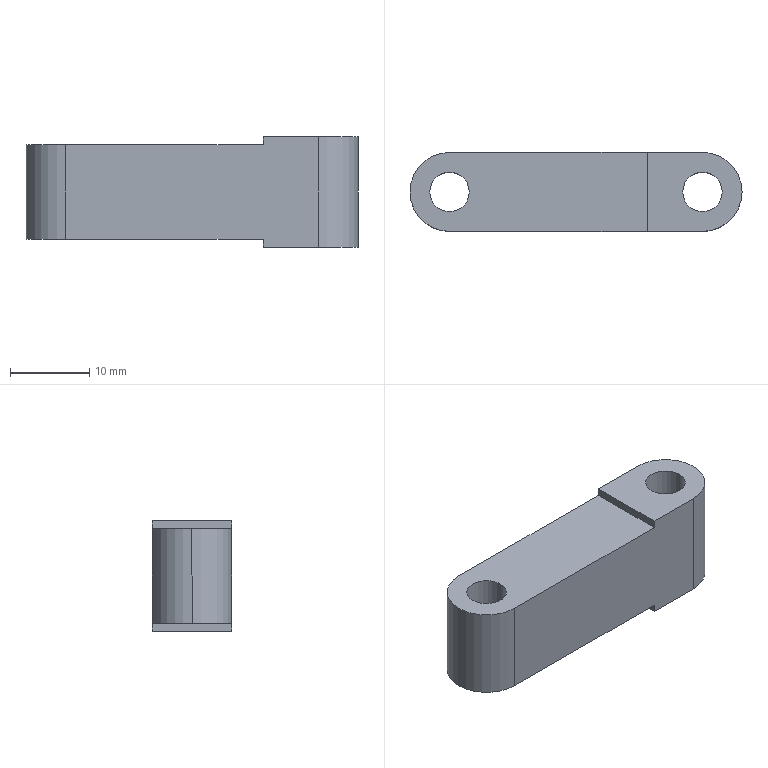Part | STEP file | gripper arm 2_default | 1 solid | 16 faces | box 42 x 10 x 14 mm | volume 4491 mm3 | cylinder 8 | plane 8 | commonest cylinder face diameters 5 x4 10 x4
STEP:
#1=CARTESIAN_POINT('',(0.,0.,0.));
#2=DIRECTION('',(0.,0.,1.));
#3=DIRECTION('',(1.,0.,0.));
#4=AXIS2_PLACEMENT_3D('',#1,#2,#3);
#5=CARTESIAN_POINT('',(18.5,0.,0.));
#6=VERTEX_POINT('',#5);
#7=CARTESIAN_POINT('',(18.5,0.,14.));
#8=VERTEX_POINT('',#7);
#9=CARTESIAN_POINT('',(18.5,0.,0.));
#10=DIRECTION('',(0.,0.,1.));
#11=VECTOR('',#10,1.);
#12=LINE('',#9,#11);
#13=CARTESIAN_POINT('',(16.,0.,0.));
#14=DIRECTION('',(0.,0.,1.));
#15=DIRECTION('',(1.,0.,0.));
#16=AXIS2_PLACEMENT_3D('',#13,#14,#15);
#17=CYLINDRICAL_SURFACE('',#16,2.5);
#18=CARTESIAN_POINT('',(6.283,0.));
#19=DIRECTION('',(0.,1.));
#20=VECTOR('',#19,1.);
#21=LINE('',#18,#20);
#22=(GEOMETRIC_REPRESENTATION_CONTEXT(2)PARAMETRIC_REPRESENTATION_CONTEXT()REPRESENTATION_CONTEXT('',''));
#23=DEFINITIONAL_REPRESENTATION('',(#21),#22);
#24=PCURVE('',#17,#23);
#25=CARTESIAN_POINT('',(16.,0.,0.));
#26=DIRECTION('',(0.,0.,1.));
#27=DIRECTION('',(1.,0.,0.));
#28=AXIS2_PLACEMENT_3D('',#25,#26,#27);
#29=CYLINDRICAL_SURFACE('',#28,2.5);
#30=CARTESIAN_POINT('',(0.,0.));
#31=DIRECTION('',(0.,1.));
#32=VECTOR('',#31,1.);
#33=LINE('',#30,#32);
#34=(GEOMETRIC_REPRESENTATION_CONTEXT(2)PARAMETRIC_REPRESENTATION_CONTEXT()REPRESENTATION_CONTEXT('',''));
#35=DEFINITIONAL_REPRESENTATION('',(#33),#34);
#36=PCURVE('',#29,#35);
#37=SURFACE_CURVE('',#12,(#24,#36),.PCURVE_S1.);
#38=EDGE_CURVE('',#6,#8,#37,.T.);
#39=ORIENTED_EDGE('',*,*,#38,.T.);
#40=CARTESIAN_POINT('',(13.5,0.,14.));
#41=VERTEX_POINT('',#40);
#42=CARTESIAN_POINT('',(16.,0.,14.));
#43=DIRECTION('',(0.,0.,1.));
#44=DIRECTION('',(1.,0.,0.));
#45=AXIS2_PLACEMENT_3D('',#42,#43,#44);
#46=CIRCLE('',#45,2.5);
#47=CARTESIAN_POINT('',(0.,14.));
#48=DIRECTION('',(1.,0.));
#49=VECTOR('',#48,1.);
#50=LINE('',#47,#49);
#51=(GEOMETRIC_REPRESENTATION_CONTEXT(2)PARAMETRIC_REPRESENTATION_CONTEXT()REPRESENTATION_CONTEXT('',''));
#52=DEFINITIONAL_REPRESENTATION('',(#50),#51);
#53=PCURVE('',#17,#52);
#54=CARTESIAN_POINT('',(0.,0.,14.));
#55=DIRECTION('',(0.,0.,1.));
#56=DIRECTION('',(1.,0.,0.));
#57=AXIS2_PLACEMENT_3D('',#54,#55,#56);
#58=PLANE('',#57);
#59=CARTESIAN_POINT('',(16.,0.));
#60=DIRECTION('',(1.,0.));
#61=AXIS2_PLACEMENT_2D('',#59,#60);
#62=CIRCLE('',#61,2.5);
#63=(GEOMETRIC_REPRESENTATION_CONTEXT(2)PARAMETRIC_REPRESENTATION_CONTEXT()REPRESENTATION_CONTEXT('',''));
#64=DEFINITIONAL_REPRESENTATION('',(#62),#63);
#65=PCURVE('',#58,#64);
#66=SURFACE_CURVE('',#46,(#53,#65),.PCURVE_S1.);
#67=EDGE_CURVE('',#41,#8,#66,.T.);
#68=ORIENTED_EDGE('',*,*,#67,.F.);
#69=CARTESIAN_POINT('',(13.5,0.,0.));
#70=VERTEX_POINT('',#69);
#71=CARTESIAN_POINT('',(13.5,0.,0.));
#72=DIRECTION('',(0.,0.,1.));
#73=VECTOR('',#72,1.);
#74=LINE('',#71,#73);
#75=CARTESIAN_POINT('',(3.142,0.));
#76=DIRECTION('',(0.,1.));
#77=VECTOR('',#76,1.);
#78=LINE('',#75,#77);
#79=(GEOMETRIC_REPRESENTATION_CONTEXT(2)PARAMETRIC_REPRESENTATION_CONTEXT()REPRESENTATION_CONTEXT('',''));
#80=DEFINITIONAL_REPRESENTATION('',(#78),#79);
#81=PCURVE('',#17,#80);
#82=CARTESIAN_POINT('',(3.142,0.));
#83=DIRECTION('',(0.,1.));
#84=VECTOR('',#83,1.);
#85=LINE('',#82,#84);
#86=(GEOMETRIC_REPRESENTATION_CONTEXT(2)PARAMETRIC_REPRESENTATION_CONTEXT()REPRESENTATION_CONTEXT('',''));
#87=DEFINITIONAL_REPRESENTATION('',(#85),#86);
#88=PCURVE('',#29,#87);
#89=SURFACE_CURVE('',#74,(#81,#88),.PCURVE_S1.);
#90=EDGE_CURVE('',#70,#41,#89,.T.);
#91=ORIENTED_EDGE('',*,*,#90,.F.);
#92=CARTESIAN_POINT('',(16.,0.,0.));
#93=DIRECTION('',(0.,0.,1.));
#94=DIRECTION('',(1.,0.,0.));
#95=AXIS2_PLACEMENT_3D('',#92,#93,#94);
#96=CIRCLE('',#95,2.5);
#97=CARTESIAN_POINT('',(0.,0.));
#98=DIRECTION('',(1.,0.));
#99=VECTOR('',#98,1.);
#100=LINE('',#97,#99);
#101=(GEOMETRIC_REPRESENTATION_CONTEXT(2)PARAMETRIC_REPRESENTATION_CONTEXT()REPRESENTATION_CONTEXT('',''));
#102=DEFINITIONAL_REPRESENTATION('',(#100),#101);
#103=PCURVE('',#17,#102);
#104=CARTESIAN_POINT('',(0.,0.,0.));
#105=DIRECTION('',(0.,0.,1.));
#106=DIRECTION('',(1.,0.,0.));
#107=AXIS2_PLACEMENT_3D('',#104,#105,#106);
#108=PLANE('',#107);
#109=CARTESIAN_POINT('',(16.,0.));
#110=DIRECTION('',(1.,0.));
#111=AXIS2_PLACEMENT_2D('',#109,#110);
#112=CIRCLE('',#111,2.5);
#113=(GEOMETRIC_REPRESENTATION_CONTEXT(2)PARAMETRIC_REPRESENTATION_CONTEXT()REPRESENTATION_CONTEXT('',''));
#114=DEFINITIONAL_REPRESENTATION('',(#112),#113);
#115=PCURVE('',#108,#114);
#116=SURFACE_CURVE('',#96,(#103,#115),.PCURVE_S1.);
#117=EDGE_CURVE('',#70,#6,#116,.T.);
#118=ORIENTED_EDGE('',*,*,#117,.T.);
#119=EDGE_LOOP('',(#39,#68,#91,#118));
#120=FACE_BOUND('',#119,.F.);
#121=ADVANCED_FACE('',(#120),#17,.F.);
#122=CARTESIAN_POINT('',(-13.5,0.,1.));
#123=VERTEX_POINT('',#122);
#124=CARTESIAN_POINT('',(-13.5,0.,13.));
#125=VERTEX_POINT('',#124);
#126=CARTESIAN_POINT('',(-13.5,0.,0.));
#127=DIRECTION('',(0.,0.,1.));
#128=VECTOR('',#127,1.);
#129=LINE('',#126,#128);
#130=CARTESIAN_POINT('',(-16.,0.,0.));
#131=DIRECTION('',(0.,0.,1.));
#132=DIRECTION('',(1.,0.,0.));
#133=AXIS2_PLACEMENT_3D('',#130,#131,#132);
#134=CYLINDRICAL_SURFACE('',#133,2.5);
#135=CARTESIAN_POINT('',(6.283,0.));
#136=DIRECTION('',(0.,1.));
#137=VECTOR('',#136,1.);
#138=LINE('',#135,#137);
#139=(GEOMETRIC_REPRESENTATION_CONTEXT(2)PARAMETRIC_REPRESENTATION_CONTEXT()REPRESENTATION_CONTEXT('',''));
#140=DEFINITIONAL_REPRESENTATION('',(#138),#139);
#141=PCURVE('',#134,#140);
#142=CARTESIAN_POINT('',(-16.,0.,0.));
#143=DIRECTION('',(0.,0.,1.));
#144=DIRECTION('',(1.,0.,0.));
#145=AXIS2_PLACEMENT_3D('',#142,#143,#144);
#146=CYLINDRICAL_SURFACE('',#145,2.5);
#147=CARTESIAN_POINT('',(0.,0.));
#148=DIRECTION('',(0.,1.));
#149=VECTOR('',#148,1.);
#150=LINE('',#147,#149);
#151=(GEOMETRIC_REPRESENTATION_CONTEXT(2)PARAMETRIC_REPRESENTATION_CONTEXT()REPRESENTATION_CONTEXT('',''));
#152=DEFINITIONAL_REPRESENTATION('',(#150),#151);
#153=PCURVE('',#146,#152);
#154=SURFACE_CURVE('',#129,(#141,#153),.PCURVE_S1.);
#155=EDGE_CURVE('',#123,#125,#154,.T.);
#156=ORIENTED_EDGE('',*,*,#155,.T.);
#157=CARTESIAN_POINT('',(-18.5,0.,13.));
#158=VERTEX_POINT('',#157);
#159=CARTESIAN_POINT('',(-16.,0.,13.));
#160=DIRECTION('',(0.,0.,-1.));
#161=DIRECTION('',(1.,0.,0.));
#162=AXIS2_PLACEMENT_3D('',#159,#160,#161);
#163=CIRCLE('',#162,2.5);
#164=CARTESIAN_POINT('',(6.283,13.));
#165=DIRECTION('',(-1.,0.));
#166=VECTOR('',#165,1.);
#167=LINE('',#164,#166);
#168=(GEOMETRIC_REPRESENTATION_CONTEXT(2)PARAMETRIC_REPRESENTATION_CONTEXT()REPRESENTATION_CONTEXT('',''));
#169=DEFINITIONAL_REPRESENTATION('',(#167),#168);
#170=PCURVE('',#134,#169);
#171=CARTESIAN_POINT('',(0.,0.,13.));
#172=DIRECTION('',(0.,0.,1.));
#173=DIRECTION('',(1.,0.,0.));
#174=AXIS2_PLACEMENT_3D('',#171,#172,#173);
#175=PLANE('',#174);
#176=CARTESIAN_POINT('',(-13.5,0.));
#177=CARTESIAN_POINT('',(-13.5,-4.33));
#178=CARTESIAN_POINT('',(-17.25,-2.165));
#179=CARTESIAN_POINT('',(-21.,0.));
#180=CARTESIAN_POINT('',(-17.25,2.165));
#181=CARTESIAN_POINT('',(-13.5,4.33));
#182=CARTESIAN_POINT('',(-13.5,0.));
#183=(BOUNDED_CURVE()B_SPLINE_CURVE(2,(#176,#177,#178,#179,#180,#181,#182),.UNSPECIFIED.,.T.,.F.)B_SPLINE_CURVE_WITH_KNOTS((1,2,2,2,2,1),(-2.094,0.,2.094,4.189,6.283,8.378),.UNSPECIFIED.)CURVE()GEOMETRIC_REPRESENTATION_ITEM()RATIONAL_B_SPLINE_CURVE((1.,0.5,1.,0.5,1.,0.5,1.))REPRESENTATION_ITEM(''));
#184=(GEOMETRIC_REPRESENTATION_CONTEXT(2)PARAMETRIC_REPRESENTATION_CONTEXT()REPRESENTATION_CONTEXT('',''));
#185=DEFINITIONAL_REPRESENTATION('',(#183),#184);
#186=PCURVE('',#175,#185);
#187=SURFACE_CURVE('',#163,(#170,#186),.PCURVE_S1.);
#188=EDGE_CURVE('',#125,#158,#187,.T.);
#189=ORIENTED_EDGE('',*,*,#188,.T.);
#190=CARTESIAN_POINT('',(-18.5,0.,1.));
#191=VERTEX_POINT('',#190);
#192=CARTESIAN_POINT('',(-18.5,0.,0.));
#193=DIRECTION('',(0.,0.,1.));
#194=VECTOR('',#193,1.);
#195=LINE('',#192,#194);
#196=CARTESIAN_POINT('',(3.142,0.));
#197=DIRECTION('',(0.,1.));
#198=VECTOR('',#197,1.);
#199=LINE('',#196,#198);
#200=(GEOMETRIC_REPRESENTATION_CONTEXT(2)PARAMETRIC_REPRESENTATION_CONTEXT()REPRESENTATION_CONTEXT('',''));
#201=DEFINITIONAL_REPRESENTATION('',(#199),#200);
#202=PCURVE('',#134,#201);
#203=CARTESIAN_POINT('',(3.142,0.));
#204=DIRECTION('',(0.,1.));
#205=VECTOR('',#204,1.);
#206=LINE('',#203,#205);
#207=(GEOMETRIC_REPRESENTATION_CONTEXT(2)PARAMETRIC_REPRESENTATION_CONTEXT()REPRESENTATION_CONTEXT('',''));
#208=DEFINITIONAL_REPRESENTATION('',(#206),#207);
#209=PCURVE('',#146,#208);
#210=SURFACE_CURVE('',#195,(#202,#209),.PCURVE_S1.);
#211=EDGE_CURVE('',#191,#158,#210,.T.);
#212=ORIENTED_EDGE('',*,*,#211,.F.);
#213=CARTESIAN_POINT('',(-16.,0.,1.));
#214=DIRECTION('',(0.,0.,1.));
#215=DIRECTION('',(-1.,0.,0.));
#216=AXIS2_PLACEMENT_3D('',#213,#214,#215);
#217=CIRCLE('',#216,2.5);
#218=CARTESIAN_POINT('',(3.142,1.));
#219=DIRECTION('',(1.,0.));
#220=VECTOR('',#219,1.);
#221=LINE('',#218,#220);
#222=(GEOMETRIC_REPRESENTATION_CONTEXT(2)PARAMETRIC_REPRESENTATION_CONTEXT()REPRESENTATION_CONTEXT('',''));
#223=DEFINITIONAL_REPRESENTATION('',(#221),#222);
#224=PCURVE('',#134,#223);
#225=CARTESIAN_POINT('',(0.,0.,1.));
#226=DIRECTION('',(0.,0.,-1.));
#227=DIRECTION('',(-1.,0.,0.));
#228=AXIS2_PLACEMENT_3D('',#225,#226,#227);
#229=PLANE('',#228);
#230=CARTESIAN_POINT('',(18.5,0.));
#231=CARTESIAN_POINT('',(18.5,-4.33));
#232=CARTESIAN_POINT('',(14.75,-2.165));
#233=CARTESIAN_POINT('',(11.,0.));
#234=CARTESIAN_POINT('',(14.75,2.165));
#235=CARTESIAN_POINT('',(18.5,4.33));
#236=CARTESIAN_POINT('',(18.5,0.));
#237=(BOUNDED_CURVE()B_SPLINE_CURVE(2,(#230,#231,#232,#233,#234,#235,#236),.UNSPECIFIED.,.T.,.F.)B_SPLINE_CURVE_WITH_KNOTS((1,2,2,2,2,1),(-2.094,0.,2.094,4.189,6.283,8.378),.UNSPECIFIED.)CURVE()GEOMETRIC_REPRESENTATION_ITEM()RATIONAL_B_SPLINE_CURVE((1.,0.5,1.,0.5,1.,0.5,1.))REPRESENTATION_ITEM(''));
#238=(GEOMETRIC_REPRESENTATION_CONTEXT(2)PARAMETRIC_REPRESENTATION_CONTEXT()REPRESENTATION_CONTEXT('',''));
#239=DEFINITIONAL_REPRESENTATION('',(#237),#238);
#240=PCURVE('',#229,#239);
#241=SURFACE_CURVE('',#217,(#224,#240),.PCURVE_S1.);
#242=EDGE_CURVE('',#191,#123,#241,.T.);
#243=ORIENTED_EDGE('',*,*,#242,.T.);
#244=EDGE_LOOP('',(#156,#189,#212,#243));
#245=FACE_BOUND('',#244,.F.);
#246=ADVANCED_FACE('',(#245),#134,.F.);
#247=CARTESIAN_POINT('',(-16.,0.,13.));
#248=DIRECTION('',(0.,0.,-1.));
#249=DIRECTION('',(1.,0.,0.));
#250=AXIS2_PLACEMENT_3D('',#247,#248,#249);
#251=CIRCLE('',#250,2.5);
#252=CARTESIAN_POINT('',(6.283,13.));
#253=DIRECTION('',(-1.,0.));
#254=VECTOR('',#253,1.);
#255=LINE('',#252,#254);
#256=(GEOMETRIC_REPRESENTATION_CONTEXT(2)PARAMETRIC_REPRESENTATION_CONTEXT()REPRESENTATION_CONTEXT('',''));
#257=DEFINITIONAL_REPRESENTATION('',(#255),#256);
#258=PCURVE('',#146,#257);
#259=CARTESIAN_POINT('',(-13.5,0.));
#260=CARTESIAN_POINT('',(-13.5,-4.33));
#261=CARTESIAN_POINT('',(-17.25,-2.165));
#262=CARTESIAN_POINT('',(-21.,0.));
#263=CARTESIAN_POINT('',(-17.25,2.165));
#264=CARTESIAN_POINT('',(-13.5,4.33));
#265=CARTESIAN_POINT('',(-13.5,0.));
#266=(BOUNDED_CURVE()B_SPLINE_CURVE(2,(#259,#260,#261,#262,#263,#264,#265),.UNSPECIFIED.,.T.,.F.)B_SPLINE_CURVE_WITH_KNOTS((1,2,2,2,2,1),(-2.094,0.,2.094,4.189,6.283,8.378),.UNSPECIFIED.)CURVE()GEOMETRIC_REPRESENTATION_ITEM()RATIONAL_B_SPLINE_CURVE((1.,0.5,1.,0.5,1.,0.5,1.))REPRESENTATION_ITEM(''));
#267=(GEOMETRIC_REPRESENTATION_CONTEXT(2)PARAMETRIC_REPRESENTATION_CONTEXT()REPRESENTATION_CONTEXT('',''));
#268=DEFINITIONAL_REPRESENTATION('',(#266),#267);
#269=PCURVE('',#175,#268);
#270=SURFACE_CURVE('',#251,(#258,#269),.PCURVE_S1.);
#271=EDGE_CURVE('',#158,#125,#270,.T.);
#272=ORIENTED_EDGE('',*,*,#271,.T.);
#273=ORIENTED_EDGE('',*,*,#155,.F.);
#274=CARTESIAN_POINT('',(-16.,0.,1.));
#275=DIRECTION('',(0.,0.,1.));
#276=DIRECTION('',(-1.,0.,0.));
#277=AXIS2_PLACEMENT_3D('',#274,#275,#276);
#278=CIRCLE('',#277,2.5);
#279=CARTESIAN_POINT('',(-3.142,1.));
#280=DIRECTION('',(1.,0.));
#281=VECTOR('',#280,1.);
#282=LINE('',#279,#281);
#283=(GEOMETRIC_REPRESENTATION_CONTEXT(2)PARAMETRIC_REPRESENTATION_CONTEXT()REPRESENTATION_CONTEXT('',''));
#284=DEFINITIONAL_REPRESENTATION('',(#282),#283);
#285=PCURVE('',#146,#284);
#286=CARTESIAN_POINT('',(18.5,0.));
#287=CARTESIAN_POINT('',(18.5,-4.33));
#288=CARTESIAN_POINT('',(14.75,-2.165));
#289=CARTESIAN_POINT('',(11.,0.));
#290=CARTESIAN_POINT('',(14.75,2.165));
#291=CARTESIAN_POINT('',(18.5,4.33));
#292=CARTESIAN_POINT('',(18.5,0.));
#293=(BOUNDED_CURVE()B_SPLINE_CURVE(2,(#286,#287,#288,#289,#290,#291,#292),.UNSPECIFIED.,.T.,.F.)B_SPLINE_CURVE_WITH_KNOTS((1,2,2,2,2,1),(-2.094,0.,2.094,4.189,6.283,8.378),.UNSPECIFIED.)CURVE()GEOMETRIC_REPRESENTATION_ITEM()RATIONAL_B_SPLINE_CURVE((1.,0.5,1.,0.5,1.,0.5,1.))REPRESENTATION_ITEM(''));
#294=(GEOMETRIC_REPRESENTATION_CONTEXT(2)PARAMETRIC_REPRESENTATION_CONTEXT()REPRESENTATION_CONTEXT('',''));
#295=DEFINITIONAL_REPRESENTATION('',(#293),#294);
#296=PCURVE('',#229,#295);
#297=SURFACE_CURVE('',#278,(#285,#296),.PCURVE_S1.);
#298=EDGE_CURVE('',#123,#191,#297,.T.);
#299=ORIENTED_EDGE('',*,*,#298,.T.);
#300=ORIENTED_EDGE('',*,*,#211,.T.);
#301=EDGE_LOOP('',(#272,#273,#299,#300));
#302=FACE_BOUND('',#301,.F.);
#303=ADVANCED_FACE('',(#302),#146,.F.);
#304=CARTESIAN_POINT('',(-16.,5.,1.));
#305=VERTEX_POINT('',#304);
#306=CARTESIAN_POINT('',(-16.,5.,13.));
#307=VERTEX_POINT('',#306);
#308=CARTESIAN_POINT('',(-16.,5.,14.));
#309=DIRECTION('',(0.,0.,1.));
#310=VECTOR('',#309,1.);
#311=LINE('',#308,#310);
#312=CARTESIAN_POINT('',(-16.,0.,14.));
#313=DIRECTION('',(0.,0.,-1.));
#314=DIRECTION('',(-1.,0.,0.));
#315=AXIS2_PLACEMENT_3D('',#312,#313,#314);
#316=CYLINDRICAL_SURFACE('',#315,5.);
#317=CARTESIAN_POINT('',(1.571,0.));
#318=DIRECTION('',(0.,-1.));
#319=VECTOR('',#318,1.);
#320=LINE('',#317,#319);
#321=(GEOMETRIC_REPRESENTATION_CONTEXT(2)PARAMETRIC_REPRESENTATION_CONTEXT()REPRESENTATION_CONTEXT('',''));
#322=DEFINITIONAL_REPRESENTATION('',(#320),#321);
#323=PCURVE('',#316,#322);
#324=CARTESIAN_POINT('',(-21.,5.,14.));
#325=DIRECTION('',(0.,-1.,0.));
#326=DIRECTION('',(0.,0.,-1.));
#327=AXIS2_PLACEMENT_3D('',#324,#325,#326);
#328=PLANE('',#327);
#329=CARTESIAN_POINT('',(0.,5.));
#330=DIRECTION('',(-1.,0.));
#331=VECTOR('',#330,1.);
#332=LINE('',#329,#331);
#333=(GEOMETRIC_REPRESENTATION_CONTEXT(2)PARAMETRIC_REPRESENTATION_CONTEXT()REPRESENTATION_CONTEXT('',''));
#334=DEFINITIONAL_REPRESENTATION('',(#332),#333);
#335=PCURVE('',#328,#334);
#336=SURFACE_CURVE('',#311,(#323,#335),.PCURVE_S1.);
#337=EDGE_CURVE('',#305,#307,#336,.T.);
#338=ORIENTED_EDGE('',*,*,#337,.F.);
#339=CARTESIAN_POINT('',(-21.,0.,1.));
#340=VERTEX_POINT('',#339);
#341=CARTESIAN_POINT('',(-16.,0.,1.));
#342=DIRECTION('',(0.,0.,1.));
#343=DIRECTION('',(-1.,0.,0.));
#344=AXIS2_PLACEMENT_3D('',#341,#342,#343);
#345=CIRCLE('',#344,5.);
#346=CARTESIAN_POINT('',(6.283,13.));
#347=DIRECTION('',(-1.,0.));
#348=VECTOR('',#347,1.);
#349=LINE('',#346,#348);
#350=(GEOMETRIC_REPRESENTATION_CONTEXT(2)PARAMETRIC_REPRESENTATION_CONTEXT()REPRESENTATION_CONTEXT('',''));
#351=DEFINITIONAL_REPRESENTATION('',(#349),#350);
#352=PCURVE('',#316,#351);
#353=CARTESIAN_POINT('',(21.,0.));
#354=CARTESIAN_POINT('',(21.,-8.66));
#355=CARTESIAN_POINT('',(13.5,-4.33));
#356=CARTESIAN_POINT('',(6.,0.));
#357=CARTESIAN_POINT('',(13.5,4.33));
#358=CARTESIAN_POINT('',(21.,8.66));
#359=CARTESIAN_POINT('',(21.,0.));
#360=(BOUNDED_CURVE()B_SPLINE_CURVE(2,(#353,#354,#355,#356,#357,#358,#359),.UNSPECIFIED.,.T.,.F.)B_SPLINE_CURVE_WITH_KNOTS((1,2,2,2,2,1),(-2.094,0.,2.094,4.189,6.283,8.378),.UNSPECIFIED.)CURVE()GEOMETRIC_REPRESENTATION_ITEM()RATIONAL_B_SPLINE_CURVE((1.,0.5,1.,0.5,1.,0.5,1.))REPRESENTATION_ITEM(''));
#361=(GEOMETRIC_REPRESENTATION_CONTEXT(2)PARAMETRIC_REPRESENTATION_CONTEXT()REPRESENTATION_CONTEXT('',''));
#362=DEFINITIONAL_REPRESENTATION('',(#360),#361);
#363=PCURVE('',#229,#362);
#364=SURFACE_CURVE('',#345,(#352,#363),.PCURVE_S1.);
#365=EDGE_CURVE('',#305,#340,#364,.T.);
#366=ORIENTED_EDGE('',*,*,#365,.T.);
#367=CARTESIAN_POINT('',(-21.,0.,13.));
#368=VERTEX_POINT('',#367);
#369=CARTESIAN_POINT('',(-21.,0.,14.));
#370=DIRECTION('',(0.,0.,-1.));
#371=VECTOR('',#370,1.);
#372=LINE('',#369,#371);
#373=CARTESIAN_POINT('',(0.,0.));
#374=DIRECTION('',(0.,1.));
#375=VECTOR('',#374,1.);
#376=LINE('',#373,#375);
#377=(GEOMETRIC_REPRESENTATION_CONTEXT(2)PARAMETRIC_REPRESENTATION_CONTEXT()REPRESENTATION_CONTEXT('',''));
#378=DEFINITIONAL_REPRESENTATION('',(#376),#377);
#379=PCURVE('',#316,#378);
#380=CARTESIAN_POINT('',(-16.,0.,14.));
#381=DIRECTION('',(0.,0.,-1.));
#382=DIRECTION('',(-1.,0.,0.));
#383=AXIS2_PLACEMENT_3D('',#380,#381,#382);
#384=CYLINDRICAL_SURFACE('',#383,5.);
#385=CARTESIAN_POINT('',(6.283,0.));
#386=DIRECTION('',(0.,1.));
#387=VECTOR('',#386,1.);
#388=LINE('',#385,#387);
#389=(GEOMETRIC_REPRESENTATION_CONTEXT(2)PARAMETRIC_REPRESENTATION_CONTEXT()REPRESENTATION_CONTEXT('',''));
#390=DEFINITIONAL_REPRESENTATION('',(#388),#389);
#391=PCURVE('',#384,#390);
#392=SURFACE_CURVE('',#372,(#379,#391),.PCURVE_S1.);
#393=EDGE_CURVE('',#368,#340,#392,.T.);
#394=ORIENTED_EDGE('',*,*,#393,.F.);
#395=CARTESIAN_POINT('',(-16.,0.,13.));
#396=DIRECTION('',(0.,0.,-1.));
#397=DIRECTION('',(1.,0.,0.));
#398=AXIS2_PLACEMENT_3D('',#395,#396,#397);
#399=CIRCLE('',#398,5.);
#400=CARTESIAN_POINT('',(-3.142,1.));
#401=DIRECTION('',(1.,0.));
#402=VECTOR('',#401,1.);
#403=LINE('',#400,#402);
#404=(GEOMETRIC_REPRESENTATION_CONTEXT(2)PARAMETRIC_REPRESENTATION_CONTEXT()REPRESENTATION_CONTEXT('',''));
#405=DEFINITIONAL_REPRESENTATION('',(#403),#404);
#406=PCURVE('',#316,#405);
#407=CARTESIAN_POINT('',(-11.,0.));
#408=CARTESIAN_POINT('',(-11.,-8.66));
#409=CARTESIAN_POINT('',(-18.5,-4.33));
#410=CARTESIAN_POINT('',(-26.,0.));
#411=CARTESIAN_POINT('',(-18.5,4.33));
#412=CARTESIAN_POINT('',(-11.,8.66));
#413=CARTESIAN_POINT('',(-11.,0.));
#414=(BOUNDED_CURVE()B_SPLINE_CURVE(2,(#407,#408,#409,#410,#411,#412,#413),.UNSPECIFIED.,.T.,.F.)B_SPLINE_CURVE_WITH_KNOTS((1,2,2,2,2,1),(-2.094,0.,2.094,4.189,6.283,8.378),.UNSPECIFIED.)CURVE()GEOMETRIC_REPRESENTATION_ITEM()RATIONAL_B_SPLINE_CURVE((1.,0.5,1.,0.5,1.,0.5,1.))REPRESENTATION_ITEM(''));
#415=(GEOMETRIC_REPRESENTATION_CONTEXT(2)PARAMETRIC_REPRESENTATION_CONTEXT()REPRESENTATION_CONTEXT('',''));
#416=DEFINITIONAL_REPRESENTATION('',(#414),#415);
#417=PCURVE('',#175,#416);
#418=SURFACE_CURVE('',#399,(#406,#417),.PCURVE_S1.);
#419=EDGE_CURVE('',#368,#307,#418,.T.);
#420=ORIENTED_EDGE('',*,*,#419,.T.);
#421=EDGE_LOOP('',(#338,#366,#394,#420));
#422=FACE_BOUND('',#421,.T.);
#423=ADVANCED_FACE('',(#422),#316,.T.);
#424=ORIENTED_EDGE('',*,*,#393,.T.);
#425=CARTESIAN_POINT('',(-16.,-5.,1.));
#426=VERTEX_POINT('',#425);
#427=CARTESIAN_POINT('',(-16.,0.,1.));
#428=DIRECTION('',(0.,0.,1.));
#429=DIRECTION('',(-1.,0.,0.));
#430=AXIS2_PLACEMENT_3D('',#427,#428,#429);
#431=CIRCLE('',#430,5.);
#432=CARTESIAN_POINT('',(6.283,13.));
#433=DIRECTION('',(-1.,0.));
#434=VECTOR('',#433,1.);
#435=LINE('',#432,#434);
#436=(GEOMETRIC_REPRESENTATION_CONTEXT(2)PARAMETRIC_REPRESENTATION_CONTEXT()REPRESENTATION_CONTEXT('',''));
#437=DEFINITIONAL_REPRESENTATION('',(#435),#436);
#438=PCURVE('',#384,#437);
#439=CARTESIAN_POINT('',(21.,0.));
#440=CARTESIAN_POINT('',(21.,-8.66));
#441=CARTESIAN_POINT('',(13.5,-4.33));
#442=CARTESIAN_POINT('',(6.,0.));
#443=CARTESIAN_POINT('',(13.5,4.33));
#444=CARTESIAN_POINT('',(21.,8.66));
#445=CARTESIAN_POINT('',(21.,0.));
#446=(BOUNDED_CURVE()B_SPLINE_CURVE(2,(#439,#440,#441,#442,#443,#444,#445),.UNSPECIFIED.,.T.,.F.)B_SPLINE_CURVE_WITH_KNOTS((1,2,2,2,2,1),(-2.094,0.,2.094,4.189,6.283,8.378),.UNSPECIFIED.)CURVE()GEOMETRIC_REPRESENTATION_ITEM()RATIONAL_B_SPLINE_CURVE((1.,0.5,1.,0.5,1.,0.5,1.))REPRESENTATION_ITEM(''));
#447=(GEOMETRIC_REPRESENTATION_CONTEXT(2)PARAMETRIC_REPRESENTATION_CONTEXT()REPRESENTATION_CONTEXT('',''));
#448=DEFINITIONAL_REPRESENTATION('',(#446),#447);
#449=PCURVE('',#229,#448);
#450=SURFACE_CURVE('',#431,(#438,#449),.PCURVE_S1.);
#451=EDGE_CURVE('',#340,#426,#450,.T.);
#452=ORIENTED_EDGE('',*,*,#451,.T.);
#453=CARTESIAN_POINT('',(-16.,-5.,13.));
#454=VERTEX_POINT('',#453);
#455=CARTESIAN_POINT('',(-16.,-5.,14.));
#456=DIRECTION('',(0.,0.,-1.));
#457=VECTOR('',#456,1.);
#458=LINE('',#455,#457);
#459=CARTESIAN_POINT('',(4.712,0.));
#460=DIRECTION('',(0.,1.));
#461=VECTOR('',#460,1.);
#462=LINE('',#459,#461);
#463=(GEOMETRIC_REPRESENTATION_CONTEXT(2)PARAMETRIC_REPRESENTATION_CONTEXT()REPRESENTATION_CONTEXT('',''));
#464=DEFINITIONAL_REPRESENTATION('',(#462),#463);
#465=PCURVE('',#384,#464);
#466=CARTESIAN_POINT('',(-21.,-5.,14.));
#467=DIRECTION('',(0.,1.,0.));
#468=DIRECTION('',(0.,0.,1.));
#469=AXIS2_PLACEMENT_3D('',#466,#467,#468);
#470=PLANE('',#469);
#471=CARTESIAN_POINT('',(0.,5.));
#472=DIRECTION('',(-1.,0.));
#473=VECTOR('',#472,1.);
#474=LINE('',#471,#473);
#475=(GEOMETRIC_REPRESENTATION_CONTEXT(2)PARAMETRIC_REPRESENTATION_CONTEXT()REPRESENTATION_CONTEXT('',''));
#476=DEFINITIONAL_REPRESENTATION('',(#474),#475);
#477=PCURVE('',#470,#476);
#478=SURFACE_CURVE('',#458,(#465,#477),.PCURVE_S1.);
#479=EDGE_CURVE('',#454,#426,#478,.T.);
#480=ORIENTED_EDGE('',*,*,#479,.F.);
#481=CARTESIAN_POINT('',(-16.,0.,13.));
#482=DIRECTION('',(0.,0.,-1.));
#483=DIRECTION('',(1.,0.,0.));
#484=AXIS2_PLACEMENT_3D('',#481,#482,#483);
#485=CIRCLE('',#484,5.);
#486=CARTESIAN_POINT('',(3.142,1.));
#487=DIRECTION('',(1.,0.));
#488=VECTOR('',#487,1.);
#489=LINE('',#486,#488);
#490=(GEOMETRIC_REPRESENTATION_CONTEXT(2)PARAMETRIC_REPRESENTATION_CONTEXT()REPRESENTATION_CONTEXT('',''));
#491=DEFINITIONAL_REPRESENTATION('',(#489),#490);
#492=PCURVE('',#384,#491);
#493=CARTESIAN_POINT('',(-11.,0.));
#494=CARTESIAN_POINT('',(-11.,-8.66));
#495=CARTESIAN_POINT('',(-18.5,-4.33));
#496=CARTESIAN_POINT('',(-26.,0.));
#497=CARTESIAN_POINT('',(-18.5,4.33));
#498=CARTESIAN_POINT('',(-11.,8.66));
#499=CARTESIAN_POINT('',(-11.,0.));
#500=(BOUNDED_CURVE()B_SPLINE_CURVE(2,(#493,#494,#495,#496,#497,#498,#499),.UNSPECIFIED.,.T.,.F.)B_SPLINE_CURVE_WITH_KNOTS((1,2,2,2,2,1),(-2.094,0.,2.094,4.189,6.283,8.378),.UNSPECIFIED.)CURVE()GEOMETRIC_REPRESENTATION_ITEM()RATIONAL_B_SPLINE_CURVE((1.,0.5,1.,0.5,1.,0.5,1.))REPRESENTATION_ITEM(''));
#501=(GEOMETRIC_REPRESENTATION_CONTEXT(2)PARAMETRIC_REPRESENTATION_CONTEXT()REPRESENTATION_CONTEXT('',''));
#502=DEFINITIONAL_REPRESENTATION('',(#500),#501);
#503=PCURVE('',#175,#502);
#504=SURFACE_CURVE('',#485,(#492,#503),.PCURVE_S1.);
#505=EDGE_CURVE('',#454,#368,#504,.T.);
#506=ORIENTED_EDGE('',*,*,#505,.T.);
#507=EDGE_LOOP('',(#424,#452,#480,#506));
#508=FACE_BOUND('',#507,.T.);
#509=ADVANCED_FACE('',(#508),#384,.T.);
#510=CARTESIAN_POINT('',(16.,5.,0.));
#511=VERTEX_POINT('',#510);
#512=CARTESIAN_POINT('',(9.,5.,0.));
#513=VERTEX_POINT('',#512);
#514=CARTESIAN_POINT('',(-21.,5.,0.));
#515=DIRECTION('',(-1.,0.,0.));
#516=VECTOR('',#515,1.);
#517=LINE('',#514,#516);
#518=CARTESIAN_POINT('',(14.,0.));
#519=DIRECTION('',(0.,-1.));
#520=VECTOR('',#519,1.);
#521=LINE('',#518,#520);
#522=(GEOMETRIC_REPRESENTATION_CONTEXT(2)PARAMETRIC_REPRESENTATION_CONTEXT()REPRESENTATION_CONTEXT('',''));
#523=DEFINITIONAL_REPRESENTATION('',(#521),#522);
#524=PCURVE('',#328,#523);
#525=CARTESIAN_POINT('',(-21.,5.));
#526=DIRECTION('',(-1.,0.));
#527=VECTOR('',#526,1.);
#528=LINE('',#525,#527);
#529=(GEOMETRIC_REPRESENTATION_CONTEXT(2)PARAMETRIC_REPRESENTATION_CONTEXT()REPRESENTATION_CONTEXT('',''));
#530=DEFINITIONAL_REPRESENTATION('',(#528),#529);
#531=PCURVE('',#108,#530);
#532=SURFACE_CURVE('',#517,(#524,#531),.PCURVE_S1.);
#533=EDGE_CURVE('',#511,#513,#532,.T.);
#534=ORIENTED_EDGE('',*,*,#533,.T.);
#535=CARTESIAN_POINT('',(9.,5.,1.));
#536=VERTEX_POINT('',#535);
#537=CARTESIAN_POINT('',(9.,5.,14.));
#538=DIRECTION('',(0.,0.,1.));
#539=VECTOR('',#538,1.);
#540=LINE('',#537,#539);
#541=CARTESIAN_POINT('',(0.,30.));
#542=DIRECTION('',(-1.,0.));
#543=VECTOR('',#542,1.);
#544=LINE('',#541,#543);
#545=(GEOMETRIC_REPRESENTATION_CONTEXT(2)PARAMETRIC_REPRESENTATION_CONTEXT()REPRESENTATION_CONTEXT('',''));
#546=DEFINITIONAL_REPRESENTATION('',(#544),#545);
#547=PCURVE('',#328,#546);
#548=CARTESIAN_POINT('',(9.,6.326,1.));
#549=DIRECTION('',(1.,0.,0.));
#550=DIRECTION('',(0.,1.,0.));
#551=AXIS2_PLACEMENT_3D('',#548,#549,#550);
#552=PLANE('',#551);
#553=CARTESIAN_POINT('',(-1.326,13.));
#554=DIRECTION('',(0.,1.));
#555=VECTOR('',#554,1.);
#556=LINE('',#553,#555);
#557=(GEOMETRIC_REPRESENTATION_CONTEXT(2)PARAMETRIC_REPRESENTATION_CONTEXT()REPRESENTATION_CONTEXT('',''));
#558=DEFINITIONAL_REPRESENTATION('',(#556),#557);
#559=PCURVE('',#552,#558);
#560=SURFACE_CURVE('',#540,(#547,#559),.PCURVE_S1.);
#561=EDGE_CURVE('',#513,#536,#560,.T.);
#562=ORIENTED_EDGE('',*,*,#561,.T.);
#563=CARTESIAN_POINT('',(-21.,5.,1.));
#564=DIRECTION('',(1.,0.,0.));
#565=VECTOR('',#564,1.);
#566=LINE('',#563,#565);
#567=CARTESIAN_POINT('',(13.,0.));
#568=DIRECTION('',(0.,1.));
#569=VECTOR('',#568,1.);
#570=LINE('',#567,#569);
#571=(GEOMETRIC_REPRESENTATION_CONTEXT(2)PARAMETRIC_REPRESENTATION_CONTEXT()REPRESENTATION_CONTEXT('',''));
#572=DEFINITIONAL_REPRESENTATION('',(#570),#571);
#573=PCURVE('',#328,#572);
#574=CARTESIAN_POINT('',(21.,5.));
#575=DIRECTION('',(-1.,0.));
#576=VECTOR('',#575,1.);
#577=LINE('',#574,#576);
#578=(GEOMETRIC_REPRESENTATION_CONTEXT(2)PARAMETRIC_REPRESENTATION_CONTEXT()REPRESENTATION_CONTEXT('',''));
#579=DEFINITIONAL_REPRESENTATION('',(#577),#578);
#580=PCURVE('',#229,#579);
#581=SURFACE_CURVE('',#566,(#573,#580),.PCURVE_S1.);
#582=EDGE_CURVE('',#305,#536,#581,.T.);
#583=ORIENTED_EDGE('',*,*,#582,.F.);
#584=ORIENTED_EDGE('',*,*,#337,.T.);
#585=CARTESIAN_POINT('',(9.,5.,13.));
#586=VERTEX_POINT('',#585);
#587=CARTESIAN_POINT('',(-21.,5.,13.));
#588=DIRECTION('',(-1.,0.,0.));
#589=VECTOR('',#588,1.);
#590=LINE('',#587,#589);
#591=CARTESIAN_POINT('',(1.,0.));
#592=DIRECTION('',(0.,-1.));
#593=VECTOR('',#592,1.);
#594=LINE('',#591,#593);
#595=(GEOMETRIC_REPRESENTATION_CONTEXT(2)PARAMETRIC_REPRESENTATION_CONTEXT()REPRESENTATION_CONTEXT('',''));
#596=DEFINITIONAL_REPRESENTATION('',(#594),#595);
#597=PCURVE('',#328,#596);
#598=CARTESIAN_POINT('',(-21.,5.));
#599=DIRECTION('',(-1.,0.));
#600=VECTOR('',#599,1.);
#601=LINE('',#598,#600);
#602=(GEOMETRIC_REPRESENTATION_CONTEXT(2)PARAMETRIC_REPRESENTATION_CONTEXT()REPRESENTATION_CONTEXT('',''));
#603=DEFINITIONAL_REPRESENTATION('',(#601),#602);
#604=PCURVE('',#175,#603);
#605=SURFACE_CURVE('',#590,(#597,#604),.PCURVE_S1.);
#606=EDGE_CURVE('',#586,#307,#605,.T.);
#607=ORIENTED_EDGE('',*,*,#606,.F.);
#608=CARTESIAN_POINT('',(9.,5.,14.));
#609=VERTEX_POINT('',#608);
#610=CARTESIAN_POINT('',(9.,5.,14.));
#611=DIRECTION('',(0.,0.,1.));
#612=VECTOR('',#611,1.);
#613=LINE('',#610,#612);
#614=CARTESIAN_POINT('',(0.,30.));
#615=DIRECTION('',(-1.,0.));
#616=VECTOR('',#615,1.);
#617=LINE('',#614,#616);
#618=(GEOMETRIC_REPRESENTATION_CONTEXT(2)PARAMETRIC_REPRESENTATION_CONTEXT()REPRESENTATION_CONTEXT('',''));
#619=DEFINITIONAL_REPRESENTATION('',(#617),#618);
#620=PCURVE('',#328,#619);
#621=CARTESIAN_POINT('',(9.,7.188,13.));
#622=DIRECTION('',(1.,0.,0.));
#623=DIRECTION('',(0.,0.,-1.));
#624=AXIS2_PLACEMENT_3D('',#621,#622,#623);
#625=PLANE('',#624);
#626=CARTESIAN_POINT('',(-1.,-2.188));
#627=DIRECTION('',(-1.,0.));
#628=VECTOR('',#627,1.);
#629=LINE('',#626,#628);
#630=(GEOMETRIC_REPRESENTATION_CONTEXT(2)PARAMETRIC_REPRESENTATION_CONTEXT()REPRESENTATION_CONTEXT('',''));
#631=DEFINITIONAL_REPRESENTATION('',(#629),#630);
#632=PCURVE('',#625,#631);
#633=SURFACE_CURVE('',#613,(#620,#632),.PCURVE_S1.);
#634=EDGE_CURVE('',#586,#609,#633,.T.);
#635=ORIENTED_EDGE('',*,*,#634,.T.);
#636=CARTESIAN_POINT('',(16.,5.,14.));
#637=VERTEX_POINT('',#636);
#638=CARTESIAN_POINT('',(-21.,5.,14.));
#639=DIRECTION('',(-1.,0.,0.));
#640=VECTOR('',#639,1.);
#641=LINE('',#638,#640);
#642=CARTESIAN_POINT('',(0.,0.));
#643=DIRECTION('',(0.,-1.));
#644=VECTOR('',#643,1.);
#645=LINE('',#642,#644);
#646=(GEOMETRIC_REPRESENTATION_CONTEXT(2)PARAMETRIC_REPRESENTATION_CONTEXT()REPRESENTATION_CONTEXT('',''));
#647=DEFINITIONAL_REPRESENTATION('',(#645),#646);
#648=PCURVE('',#328,#647);
#649=CARTESIAN_POINT('',(-21.,5.));
#650=DIRECTION('',(-1.,0.));
#651=VECTOR('',#650,1.);
#652=LINE('',#649,#651);
#653=(GEOMETRIC_REPRESENTATION_CONTEXT(2)PARAMETRIC_REPRESENTATION_CONTEXT()REPRESENTATION_CONTEXT('',''));
#654=DEFINITIONAL_REPRESENTATION('',(#652),#653);
#655=PCURVE('',#58,#654);
#656=SURFACE_CURVE('',#641,(#648,#655),.PCURVE_S1.);
#657=EDGE_CURVE('',#637,#609,#656,.T.);
#658=ORIENTED_EDGE('',*,*,#657,.F.);
#659=CARTESIAN_POINT('',(16.,5.,14.));
#660=DIRECTION('',(0.,0.,-1.));
#661=VECTOR('',#660,1.);
#662=LINE('',#659,#661);
#663=CARTESIAN_POINT('',(0.,37.));
#664=DIRECTION('',(1.,0.));
#665=VECTOR('',#664,1.);
#666=LINE('',#663,#665);
#667=(GEOMETRIC_REPRESENTATION_CONTEXT(2)PARAMETRIC_REPRESENTATION_CONTEXT()REPRESENTATION_CONTEXT('',''));
#668=DEFINITIONAL_REPRESENTATION('',(#666),#667);
#669=PCURVE('',#328,#668);
#670=CARTESIAN_POINT('',(16.,0.,14.));
#671=DIRECTION('',(0.,0.,-1.));
#672=DIRECTION('',(-1.,0.,0.));
#673=AXIS2_PLACEMENT_3D('',#670,#671,#672);
#674=CYLINDRICAL_SURFACE('',#673,5.);
#675=CARTESIAN_POINT('',(1.571,0.));
#676=DIRECTION('',(0.,1.));
#677=VECTOR('',#676,1.);
#678=LINE('',#675,#677);
#679=(GEOMETRIC_REPRESENTATION_CONTEXT(2)PARAMETRIC_REPRESENTATION_CONTEXT()REPRESENTATION_CONTEXT('',''));
#680=DEFINITIONAL_REPRESENTATION('',(#678),#679);
#681=PCURVE('',#674,#680);
#682=SURFACE_CURVE('',#662,(#669,#681),.PCURVE_S1.);
#683=EDGE_CURVE('',#637,#511,#682,.T.);
#684=ORIENTED_EDGE('',*,*,#683,.T.);
#685=EDGE_LOOP('',(#534,#562,#583,#584,#607,#635,#658,#684));
#686=FACE_BOUND('',#685,.T.);
#687=ADVANCED_FACE('',(#686),#328,.F.);
#688=CARTESIAN_POINT('',(9.,-5.,1.));
#689=VERTEX_POINT('',#688);
#690=CARTESIAN_POINT('',(-21.,-5.,1.));
#691=DIRECTION('',(-1.,0.,0.));
#692=VECTOR('',#691,1.);
#693=LINE('',#690,#692);
#694=CARTESIAN_POINT('',(-13.,0.));
#695=DIRECTION('',(0.,-1.));
#696=VECTOR('',#695,1.);
#697=LINE('',#694,#696);
#698=(GEOMETRIC_REPRESENTATION_CONTEXT(2)PARAMETRIC_REPRESENTATION_CONTEXT()REPRESENTATION_CONTEXT('',''));
#699=DEFINITIONAL_REPRESENTATION('',(#697),#698);
#700=PCURVE('',#470,#699);
#701=CARTESIAN_POINT('',(21.,-5.));
#702=DIRECTION('',(1.,0.));
#703=VECTOR('',#702,1.);
#704=LINE('',#701,#703);
#705=(GEOMETRIC_REPRESENTATION_CONTEXT(2)PARAMETRIC_REPRESENTATION_CONTEXT()REPRESENTATION_CONTEXT('',''));
#706=DEFINITIONAL_REPRESENTATION('',(#704),#705);
#707=PCURVE('',#229,#706);
#708=SURFACE_CURVE('',#693,(#700,#707),.PCURVE_S1.);
#709=EDGE_CURVE('',#689,#426,#708,.T.);
#710=ORIENTED_EDGE('',*,*,#709,.F.);
#711=CARTESIAN_POINT('',(9.,-5.,0.));
#712=VERTEX_POINT('',#711);
#713=CARTESIAN_POINT('',(9.,-5.,14.));
#714=DIRECTION('',(0.,0.,-1.));
#715=VECTOR('',#714,1.);
#716=LINE('',#713,#715);
#717=CARTESIAN_POINT('',(0.,30.));
#718=DIRECTION('',(-1.,0.));
#719=VECTOR('',#718,1.);
#720=LINE('',#717,#719);
#721=(GEOMETRIC_REPRESENTATION_CONTEXT(2)PARAMETRIC_REPRESENTATION_CONTEXT()REPRESENTATION_CONTEXT('',''));
#722=DEFINITIONAL_REPRESENTATION('',(#720),#721);
#723=PCURVE('',#470,#722);
#724=CARTESIAN_POINT('',(-11.326,13.));
#725=DIRECTION('',(0.,-1.));
#726=VECTOR('',#725,1.);
#727=LINE('',#724,#726);
#728=(GEOMETRIC_REPRESENTATION_CONTEXT(2)PARAMETRIC_REPRESENTATION_CONTEXT()REPRESENTATION_CONTEXT('',''));
#729=DEFINITIONAL_REPRESENTATION('',(#727),#728);
#730=PCURVE('',#552,#729);
#731=SURFACE_CURVE('',#716,(#723,#730),.PCURVE_S1.);
#732=EDGE_CURVE('',#689,#712,#731,.T.);
#733=ORIENTED_EDGE('',*,*,#732,.T.);
#734=CARTESIAN_POINT('',(16.,-5.,0.));
#735=VERTEX_POINT('',#734);
#736=CARTESIAN_POINT('',(-21.,-5.,0.));
#737=DIRECTION('',(1.,0.,0.));
#738=VECTOR('',#737,1.);
#739=LINE('',#736,#738);
#740=CARTESIAN_POINT('',(-14.,0.));
#741=DIRECTION('',(0.,1.));
#742=VECTOR('',#741,1.);
#743=LINE('',#740,#742);
#744=(GEOMETRIC_REPRESENTATION_CONTEXT(2)PARAMETRIC_REPRESENTATION_CONTEXT()REPRESENTATION_CONTEXT('',''));
#745=DEFINITIONAL_REPRESENTATION('',(#743),#744);
#746=PCURVE('',#470,#745);
#747=CARTESIAN_POINT('',(-21.,-5.));
#748=DIRECTION('',(1.,0.));
#749=VECTOR('',#748,1.);
#750=LINE('',#747,#749);
#751=(GEOMETRIC_REPRESENTATION_CONTEXT(2)PARAMETRIC_REPRESENTATION_CONTEXT()REPRESENTATION_CONTEXT('',''));
#752=DEFINITIONAL_REPRESENTATION('',(#750),#751);
#753=PCURVE('',#108,#752);
#754=SURFACE_CURVE('',#739,(#746,#753),.PCURVE_S1.);
#755=EDGE_CURVE('',#712,#735,#754,.T.);
#756=ORIENTED_EDGE('',*,*,#755,.T.);
#757=CARTESIAN_POINT('',(16.,-5.,14.));
#758=VERTEX_POINT('',#757);
#759=CARTESIAN_POINT('',(16.,-5.,14.));
#760=DIRECTION('',(0.,0.,1.));
#761=VECTOR('',#760,1.);
#762=LINE('',#759,#761);
#763=CARTESIAN_POINT('',(0.,37.));
#764=DIRECTION('',(1.,0.));
#765=VECTOR('',#764,1.);
#766=LINE('',#763,#765);
#767=(GEOMETRIC_REPRESENTATION_CONTEXT(2)PARAMETRIC_REPRESENTATION_CONTEXT()REPRESENTATION_CONTEXT('',''));
#768=DEFINITIONAL_REPRESENTATION('',(#766),#767);
#769=PCURVE('',#470,#768);
#770=CARTESIAN_POINT('',(16.,0.,14.));
#771=DIRECTION('',(0.,0.,-1.));
#772=DIRECTION('',(-1.,0.,0.));
#773=AXIS2_PLACEMENT_3D('',#770,#771,#772);
#774=CYLINDRICAL_SURFACE('',#773,5.);
#775=CARTESIAN_POINT('',(4.712,0.));
#776=DIRECTION('',(0.,-1.));
#777=VECTOR('',#776,1.);
#778=LINE('',#775,#777);
#779=(GEOMETRIC_REPRESENTATION_CONTEXT(2)PARAMETRIC_REPRESENTATION_CONTEXT()REPRESENTATION_CONTEXT('',''));
#780=DEFINITIONAL_REPRESENTATION('',(#778),#779);
#781=PCURVE('',#774,#780);
#782=SURFACE_CURVE('',#762,(#769,#781),.PCURVE_S1.);
#783=EDGE_CURVE('',#735,#758,#782,.T.);
#784=ORIENTED_EDGE('',*,*,#783,.T.);
#785=CARTESIAN_POINT('',(9.,-5.,14.));
#786=VERTEX_POINT('',#785);
#787=CARTESIAN_POINT('',(-21.,-5.,14.));
#788=DIRECTION('',(1.,0.,0.));
#789=VECTOR('',#788,1.);
#790=LINE('',#787,#789);
#791=CARTESIAN_POINT('',(0.,0.));
#792=DIRECTION('',(0.,1.));
#793=VECTOR('',#792,1.);
#794=LINE('',#791,#793);
#795=(GEOMETRIC_REPRESENTATION_CONTEXT(2)PARAMETRIC_REPRESENTATION_CONTEXT()REPRESENTATION_CONTEXT('',''));
#796=DEFINITIONAL_REPRESENTATION('',(#794),#795);
#797=PCURVE('',#470,#796);
#798=CARTESIAN_POINT('',(-21.,-5.));
#799=DIRECTION('',(1.,0.));
#800=VECTOR('',#799,1.);
#801=LINE('',#798,#800);
#802=(GEOMETRIC_REPRESENTATION_CONTEXT(2)PARAMETRIC_REPRESENTATION_CONTEXT()REPRESENTATION_CONTEXT('',''));
#803=DEFINITIONAL_REPRESENTATION('',(#801),#802);
#804=PCURVE('',#58,#803);
#805=SURFACE_CURVE('',#790,(#797,#804),.PCURVE_S1.);
#806=EDGE_CURVE('',#786,#758,#805,.T.);
#807=ORIENTED_EDGE('',*,*,#806,.F.);
#808=CARTESIAN_POINT('',(9.,-5.,13.));
#809=VERTEX_POINT('',#808);
#810=CARTESIAN_POINT('',(9.,-5.,14.));
#811=DIRECTION('',(0.,0.,-1.));
#812=VECTOR('',#811,1.);
#813=LINE('',#810,#812);
#814=CARTESIAN_POINT('',(0.,30.));
#815=DIRECTION('',(-1.,0.));
#816=VECTOR('',#815,1.);
#817=LINE('',#814,#816);
#818=(GEOMETRIC_REPRESENTATION_CONTEXT(2)PARAMETRIC_REPRESENTATION_CONTEXT()REPRESENTATION_CONTEXT('',''));
#819=DEFINITIONAL_REPRESENTATION('',(#817),#818);
#820=PCURVE('',#470,#819);
#821=CARTESIAN_POINT('',(-1.,-12.188));
#822=DIRECTION('',(1.,0.));
#823=VECTOR('',#822,1.);
#824=LINE('',#821,#823);
#825=(GEOMETRIC_REPRESENTATION_CONTEXT(2)PARAMETRIC_REPRESENTATION_CONTEXT()REPRESENTATION_CONTEXT('',''));
#826=DEFINITIONAL_REPRESENTATION('',(#824),#825);
#827=PCURVE('',#625,#826);
#828=SURFACE_CURVE('',#813,(#820,#827),.PCURVE_S1.);
#829=EDGE_CURVE('',#786,#809,#828,.T.);
#830=ORIENTED_EDGE('',*,*,#829,.T.);
#831=CARTESIAN_POINT('',(-21.,-5.,13.));
#832=DIRECTION('',(1.,0.,0.));
#833=VECTOR('',#832,1.);
#834=LINE('',#831,#833);
#835=CARTESIAN_POINT('',(-1.,0.));
#836=DIRECTION('',(0.,1.));
#837=VECTOR('',#836,1.);
#838=LINE('',#835,#837);
#839=(GEOMETRIC_REPRESENTATION_CONTEXT(2)PARAMETRIC_REPRESENTATION_CONTEXT()REPRESENTATION_CONTEXT('',''));
#840=DEFINITIONAL_REPRESENTATION('',(#838),#839);
#841=PCURVE('',#470,#840);
#842=CARTESIAN_POINT('',(-21.,-5.));
#843=DIRECTION('',(1.,0.));
#844=VECTOR('',#843,1.);
#845=LINE('',#842,#844);
#846=(GEOMETRIC_REPRESENTATION_CONTEXT(2)PARAMETRIC_REPRESENTATION_CONTEXT()REPRESENTATION_CONTEXT('',''));
#847=DEFINITIONAL_REPRESENTATION('',(#845),#846);
#848=PCURVE('',#175,#847);
#849=SURFACE_CURVE('',#834,(#841,#848),.PCURVE_S1.);
#850=EDGE_CURVE('',#454,#809,#849,.T.);
#851=ORIENTED_EDGE('',*,*,#850,.F.);
#852=ORIENTED_EDGE('',*,*,#479,.T.);
#853=EDGE_LOOP('',(#710,#733,#756,#784,#807,#830,#851,#852));
#854=FACE_BOUND('',#853,.T.);
#855=ADVANCED_FACE('',(#854),#470,.F.);
#856=CARTESIAN_POINT('',(9.,7.188,14.));
#857=DIRECTION('',(0.,1.,0.));
#858=VECTOR('',#857,1.);
#859=LINE('',#856,#858);
#860=CARTESIAN_POINT('',(9.,7.188));
#861=DIRECTION('',(0.,1.));
#862=VECTOR('',#861,1.);
#863=LINE('',#860,#862);
#864=(GEOMETRIC_REPRESENTATION_CONTEXT(2)PARAMETRIC_REPRESENTATION_CONTEXT()REPRESENTATION_CONTEXT('',''));
#865=DEFINITIONAL_REPRESENTATION('',(#863),#864);
#866=PCURVE('',#58,#865);
#867=CARTESIAN_POINT('',(-1.,0.));
#868=DIRECTION('',(0.,1.));
#869=VECTOR('',#868,1.);
#870=LINE('',#867,#869);
#871=(GEOMETRIC_REPRESENTATION_CONTEXT(2)PARAMETRIC_REPRESENTATION_CONTEXT()REPRESENTATION_CONTEXT('',''));
#872=DEFINITIONAL_REPRESENTATION('',(#870),#871);
#873=PCURVE('',#625,#872);
#874=SURFACE_CURVE('',#859,(#866,#873),.PCURVE_S1.);
#875=EDGE_CURVE('',#786,#609,#874,.T.);
#876=ORIENTED_EDGE('',*,*,#875,.F.);
#877=ORIENTED_EDGE('',*,*,#806,.T.);
#878=CARTESIAN_POINT('',(21.,0.,14.));
#879=VERTEX_POINT('',#878);
#880=CARTESIAN_POINT('',(16.,0.,14.));
#881=DIRECTION('',(0.,0.,1.));
#882=DIRECTION('',(1.,0.,0.));
#883=AXIS2_PLACEMENT_3D('',#880,#881,#882);
#884=CIRCLE('',#883,5.);
#885=CARTESIAN_POINT('',(16.,0.));
#886=DIRECTION('',(1.,0.));
#887=AXIS2_PLACEMENT_2D('',#885,#886);
#888=CIRCLE('',#887,5.);
#889=(GEOMETRIC_REPRESENTATION_CONTEXT(2)PARAMETRIC_REPRESENTATION_CONTEXT()REPRESENTATION_CONTEXT('',''));
#890=DEFINITIONAL_REPRESENTATION('',(#888),#889);
#891=PCURVE('',#58,#890);
#892=CARTESIAN_POINT('',(9.425,0.));
#893=DIRECTION('',(-1.,0.));
#894=VECTOR('',#893,1.);
#895=LINE('',#892,#894);
#896=(GEOMETRIC_REPRESENTATION_CONTEXT(2)PARAMETRIC_REPRESENTATION_CONTEXT()REPRESENTATION_CONTEXT('',''));
#897=DEFINITIONAL_REPRESENTATION('',(#895),#896);
#898=PCURVE('',#774,#897);
#899=SURFACE_CURVE('',#884,(#891,#898),.PCURVE_S1.);
#900=EDGE_CURVE('',#758,#879,#899,.T.);
#901=ORIENTED_EDGE('',*,*,#900,.T.);
#902=CARTESIAN_POINT('',(16.,0.,14.));
#903=DIRECTION('',(0.,0.,1.));
#904=DIRECTION('',(1.,0.,0.));
#905=AXIS2_PLACEMENT_3D('',#902,#903,#904);
#906=CIRCLE('',#905,5.);
#907=CARTESIAN_POINT('',(16.,0.));
#908=DIRECTION('',(1.,0.));
#909=AXIS2_PLACEMENT_2D('',#907,#908);
#910=CIRCLE('',#909,5.);
#911=(GEOMETRIC_REPRESENTATION_CONTEXT(2)PARAMETRIC_REPRESENTATION_CONTEXT()REPRESENTATION_CONTEXT('',''));
#912=DEFINITIONAL_REPRESENTATION('',(#910),#911);
#913=PCURVE('',#58,#912);
#914=CARTESIAN_POINT('',(3.142,0.));
#915=DIRECTION('',(-1.,0.));
#916=VECTOR('',#915,1.);
#917=LINE('',#914,#916);
#918=(GEOMETRIC_REPRESENTATION_CONTEXT(2)PARAMETRIC_REPRESENTATION_CONTEXT()REPRESENTATION_CONTEXT('',''));
#919=DEFINITIONAL_REPRESENTATION('',(#917),#918);
#920=PCURVE('',#674,#919);
#921=SURFACE_CURVE('',#906,(#913,#920),.PCURVE_S1.);
#922=EDGE_CURVE('',#879,#637,#921,.T.);
#923=ORIENTED_EDGE('',*,*,#922,.T.);
#924=ORIENTED_EDGE('',*,*,#657,.T.);
#925=EDGE_LOOP('',(#876,#877,#901,#923,#924));
#926=FACE_BOUND('',#925,.T.);
#927=CARTESIAN_POINT('',(16.,0.,14.));
#928=DIRECTION('',(0.,0.,1.));
#929=DIRECTION('',(1.,0.,0.));
#930=AXIS2_PLACEMENT_3D('',#927,#928,#929);
#931=CIRCLE('',#930,2.5);
#932=CARTESIAN_POINT('',(16.,0.));
#933=DIRECTION('',(1.,0.));
#934=AXIS2_PLACEMENT_2D('',#932,#933);
#935=CIRCLE('',#934,2.5);
#936=(GEOMETRIC_REPRESENTATION_CONTEXT(2)PARAMETRIC_REPRESENTATION_CONTEXT()REPRESENTATION_CONTEXT('',''));
#937=DEFINITIONAL_REPRESENTATION('',(#935),#936);
#938=PCURVE('',#58,#937);
#939=CARTESIAN_POINT('',(0.,14.));
#940=DIRECTION('',(1.,0.));
#941=VECTOR('',#940,1.);
#942=LINE('',#939,#941);
#943=(GEOMETRIC_REPRESENTATION_CONTEXT(2)PARAMETRIC_REPRESENTATION_CONTEXT()REPRESENTATION_CONTEXT('',''));
#944=DEFINITIONAL_REPRESENTATION('',(#942),#943);
#945=PCURVE('',#29,#944);
#946=SURFACE_CURVE('',#931,(#938,#945),.PCURVE_S1.);
#947=EDGE_CURVE('',#8,#41,#946,.T.);
#948=ORIENTED_EDGE('',*,*,#947,.F.);
#949=ORIENTED_EDGE('',*,*,#67,.F.);
#950=EDGE_LOOP('',(#948,#949));
#951=FACE_BOUND('',#950,.T.);
#952=ADVANCED_FACE('',(#926,#951),#58,.T.);
#953=CARTESIAN_POINT('',(16.,0.,0.));
#954=DIRECTION('',(0.,0.,1.));
#955=DIRECTION('',(1.,0.,0.));
#956=AXIS2_PLACEMENT_3D('',#953,#954,#955);
#957=CIRCLE('',#956,2.5);
#958=CARTESIAN_POINT('',(16.,0.));
#959=DIRECTION('',(1.,0.));
#960=AXIS2_PLACEMENT_2D('',#958,#959);
#961=CIRCLE('',#960,2.5);
#962=(GEOMETRIC_REPRESENTATION_CONTEXT(2)PARAMETRIC_REPRESENTATION_CONTEXT()REPRESENTATION_CONTEXT('',''));
#963=DEFINITIONAL_REPRESENTATION('',(#961),#962);
#964=PCURVE('',#108,#963);
#965=CARTESIAN_POINT('',(0.,0.));
#966=DIRECTION('',(1.,0.));
#967=VECTOR('',#966,1.);
#968=LINE('',#965,#967);
#969=(GEOMETRIC_REPRESENTATION_CONTEXT(2)PARAMETRIC_REPRESENTATION_CONTEXT()REPRESENTATION_CONTEXT('',''));
#970=DEFINITIONAL_REPRESENTATION('',(#968),#969);
#971=PCURVE('',#29,#970);
#972=SURFACE_CURVE('',#957,(#964,#971),.PCURVE_S1.);
#973=EDGE_CURVE('',#6,#70,#972,.T.);
#974=ORIENTED_EDGE('',*,*,#973,.T.);
#975=ORIENTED_EDGE('',*,*,#117,.T.);
#976=EDGE_LOOP('',(#974,#975));
#977=FACE_BOUND('',#976,.T.);
#978=ORIENTED_EDGE('',*,*,#755,.F.);
#979=CARTESIAN_POINT('',(9.,0.,0.));
#980=DIRECTION('',(0.,1.,0.));
#981=VECTOR('',#980,1.);
#982=LINE('',#979,#981);
#983=CARTESIAN_POINT('',(9.,0.));
#984=DIRECTION('',(0.,1.));
#985=VECTOR('',#984,1.);
#986=LINE('',#983,#985);
#987=(GEOMETRIC_REPRESENTATION_CONTEXT(2)PARAMETRIC_REPRESENTATION_CONTEXT()REPRESENTATION_CONTEXT('',''));
#988=DEFINITIONAL_REPRESENTATION('',(#986),#987);
#989=PCURVE('',#108,#988);
#990=CARTESIAN_POINT('',(-6.326,-1.));
#991=DIRECTION('',(1.,0.));
#992=VECTOR('',#991,1.);
#993=LINE('',#990,#992);
#994=(GEOMETRIC_REPRESENTATION_CONTEXT(2)PARAMETRIC_REPRESENTATION_CONTEXT()REPRESENTATION_CONTEXT('',''));
#995=DEFINITIONAL_REPRESENTATION('',(#993),#994);
#996=PCURVE('',#552,#995);
#997=SURFACE_CURVE('',#982,(#989,#996),.PCURVE_S1.);
#998=EDGE_CURVE('',#712,#513,#997,.T.);
#999=ORIENTED_EDGE('',*,*,#998,.T.);
#1000=ORIENTED_EDGE('',*,*,#533,.F.);
#1001=CARTESIAN_POINT('',(21.,0.,0.));
#1002=VERTEX_POINT('',#1001);
#1003=CARTESIAN_POINT('',(16.,0.,0.));
#1004=DIRECTION('',(0.,0.,-1.));
#1005=DIRECTION('',(1.,0.,0.));
#1006=AXIS2_PLACEMENT_3D('',#1003,#1004,#1005);
#1007=CIRCLE('',#1006,5.);
#1008=CARTESIAN_POINT('',(21.,0.));
#1009=CARTESIAN_POINT('',(21.,-8.66));
#1010=CARTESIAN_POINT('',(13.5,-4.33));
#1011=CARTESIAN_POINT('',(6.,0.));
#1012=CARTESIAN_POINT('',(13.5,4.33));
#1013=CARTESIAN_POINT('',(21.,8.66));
#1014=CARTESIAN_POINT('',(21.,0.));
#1015=(BOUNDED_CURVE()B_SPLINE_CURVE(2,(#1008,#1009,#1010,#1011,#1012,#1013,#1014),.UNSPECIFIED.,.T.,.F.)B_SPLINE_CURVE_WITH_KNOTS((1,2,2,2,2,1),(-2.094,0.,2.094,4.189,6.283,8.378),.UNSPECIFIED.)CURVE()GEOMETRIC_REPRESENTATION_ITEM()RATIONAL_B_SPLINE_CURVE((1.,0.5,1.,0.5,1.,0.5,1.))REPRESENTATION_ITEM(''));
#1016=(GEOMETRIC_REPRESENTATION_CONTEXT(2)PARAMETRIC_REPRESENTATION_CONTEXT()REPRESENTATION_CONTEXT('',''));
#1017=DEFINITIONAL_REPRESENTATION('',(#1015),#1016);
#1018=PCURVE('',#108,#1017);
#1019=CARTESIAN_POINT('',(-3.142,14.));
#1020=DIRECTION('',(1.,0.));
#1021=VECTOR('',#1020,1.);
#1022=LINE('',#1019,#1021);
#1023=(GEOMETRIC_REPRESENTATION_CONTEXT(2)PARAMETRIC_REPRESENTATION_CONTEXT()REPRESENTATION_CONTEXT('',''));
#1024=DEFINITIONAL_REPRESENTATION('',(#1022),#1023);
#1025=PCURVE('',#674,#1024);
#1026=SURFACE_CURVE('',#1007,(#1018,#1025),.PCURVE_S1.);
#1027=EDGE_CURVE('',#511,#1002,#1026,.T.);
#1028=ORIENTED_EDGE('',*,*,#1027,.T.);
#1029=CARTESIAN_POINT('',(16.,0.,0.));
#1030=DIRECTION('',(0.,0.,-1.));
#1031=DIRECTION('',(1.,0.,0.));
#1032=AXIS2_PLACEMENT_3D('',#1029,#1030,#1031);
#1033=CIRCLE('',#1032,5.);
#1034=CARTESIAN_POINT('',(21.,0.));
#1035=CARTESIAN_POINT('',(21.,-8.66));
#1036=CARTESIAN_POINT('',(13.5,-4.33));
#1037=CARTESIAN_POINT('',(6.,0.));
#1038=CARTESIAN_POINT('',(13.5,4.33));
#1039=CARTESIAN_POINT('',(21.,8.66));
#1040=CARTESIAN_POINT('',(21.,0.));
#1041=(BOUNDED_CURVE()B_SPLINE_CURVE(2,(#1034,#1035,#1036,#1037,#1038,#1039,#1040),.UNSPECIFIED.,.T.,.F.)B_SPLINE_CURVE_WITH_KNOTS((1,2,2,2,2,1),(-2.094,0.,2.094,4.189,6.283,8.378),.UNSPECIFIED.)CURVE()GEOMETRIC_REPRESENTATION_ITEM()RATIONAL_B_SPLINE_CURVE((1.,0.5,1.,0.5,1.,0.5,1.))REPRESENTATION_ITEM(''));
#1042=(GEOMETRIC_REPRESENTATION_CONTEXT(2)PARAMETRIC_REPRESENTATION_CONTEXT()REPRESENTATION_CONTEXT('',''));
#1043=DEFINITIONAL_REPRESENTATION('',(#1041),#1042);
#1044=PCURVE('',#108,#1043);
#1045=CARTESIAN_POINT('',(3.142,14.));
#1046=DIRECTION('',(1.,0.));
#1047=VECTOR('',#1046,1.);
#1048=LINE('',#1045,#1047);
#1049=(GEOMETRIC_REPRESENTATION_CONTEXT(2)PARAMETRIC_REPRESENTATION_CONTEXT()REPRESENTATION_CONTEXT('',''));
#1050=DEFINITIONAL_REPRESENTATION('',(#1048),#1049);
#1051=PCURVE('',#774,#1050);
#1052=SURFACE_CURVE('',#1033,(#1044,#1051),.PCURVE_S1.);
#1053=EDGE_CURVE('',#1002,#735,#1052,.T.);
#1054=ORIENTED_EDGE('',*,*,#1053,.T.);
#1055=EDGE_LOOP('',(#978,#999,#1000,#1028,#1054));
#1056=FACE_BOUND('',#1055,.T.);
#1057=ADVANCED_FACE('',(#977,#1056),#108,.F.);
#1058=ORIENTED_EDGE('',*,*,#947,.F.);
#1059=ORIENTED_EDGE('',*,*,#38,.F.);
#1060=ORIENTED_EDGE('',*,*,#973,.T.);
#1061=ORIENTED_EDGE('',*,*,#90,.T.);
#1062=EDGE_LOOP('',(#1058,#1059,#1060,#1061));
#1063=FACE_BOUND('',#1062,.F.);
#1064=ADVANCED_FACE('',(#1063),#29,.F.);
#1065=ORIENTED_EDGE('',*,*,#683,.F.);
#1066=ORIENTED_EDGE('',*,*,#922,.F.);
#1067=CARTESIAN_POINT('',(21.,0.,14.));
#1068=DIRECTION('',(0.,0.,1.));
#1069=VECTOR('',#1068,1.);
#1070=LINE('',#1067,#1069);
#1071=CARTESIAN_POINT('',(3.142,0.));
#1072=DIRECTION('',(0.,-1.));
#1073=VECTOR('',#1072,1.);
#1074=LINE('',#1071,#1073);
#1075=(GEOMETRIC_REPRESENTATION_CONTEXT(2)PARAMETRIC_REPRESENTATION_CONTEXT()REPRESENTATION_CONTEXT('',''));
#1076=DEFINITIONAL_REPRESENTATION('',(#1074),#1075);
#1077=PCURVE('',#674,#1076);
#1078=CARTESIAN_POINT('',(3.142,0.));
#1079=DIRECTION('',(0.,-1.));
#1080=VECTOR('',#1079,1.);
#1081=LINE('',#1078,#1080);
#1082=(GEOMETRIC_REPRESENTATION_CONTEXT(2)PARAMETRIC_REPRESENTATION_CONTEXT()REPRESENTATION_CONTEXT('',''));
#1083=DEFINITIONAL_REPRESENTATION('',(#1081),#1082);
#1084=PCURVE('',#774,#1083);
#1085=SURFACE_CURVE('',#1070,(#1077,#1084),.PCURVE_S1.);
#1086=EDGE_CURVE('',#1002,#879,#1085,.T.);
#1087=ORIENTED_EDGE('',*,*,#1086,.F.);
#1088=ORIENTED_EDGE('',*,*,#1027,.F.);
#1089=EDGE_LOOP('',(#1065,#1066,#1087,#1088));
#1090=FACE_BOUND('',#1089,.T.);
#1091=ADVANCED_FACE('',(#1090),#674,.T.);
#1092=ORIENTED_EDGE('',*,*,#900,.F.);
#1093=ORIENTED_EDGE('',*,*,#783,.F.);
#1094=ORIENTED_EDGE('',*,*,#1053,.F.);
#1095=ORIENTED_EDGE('',*,*,#1086,.T.);
#1096=EDGE_LOOP('',(#1092,#1093,#1094,#1095));
#1097=FACE_BOUND('',#1096,.T.);
#1098=ADVANCED_FACE('',(#1097),#774,.T.);
#1099=CARTESIAN_POINT('',(9.,7.188,13.));
#1100=DIRECTION('',(0.,1.,0.));
#1101=VECTOR('',#1100,1.);
#1102=LINE('',#1099,#1101);
#1103=CARTESIAN_POINT('',(0.,0.));
#1104=DIRECTION('',(0.,1.));
#1105=VECTOR('',#1104,1.);
#1106=LINE('',#1103,#1105);
#1107=(GEOMETRIC_REPRESENTATION_CONTEXT(2)PARAMETRIC_REPRESENTATION_CONTEXT()REPRESENTATION_CONTEXT('',''));
#1108=DEFINITIONAL_REPRESENTATION('',(#1106),#1107);
#1109=PCURVE('',#625,#1108);
#1110=CARTESIAN_POINT('',(9.,7.188));
#1111=DIRECTION('',(0.,1.));
#1112=VECTOR('',#1111,1.);
#1113=LINE('',#1110,#1112);
#1114=(GEOMETRIC_REPRESENTATION_CONTEXT(2)PARAMETRIC_REPRESENTATION_CONTEXT()REPRESENTATION_CONTEXT('',''));
#1115=DEFINITIONAL_REPRESENTATION('',(#1113),#1114);
#1116=PCURVE('',#175,#1115);
#1117=SURFACE_CURVE('',#1102,(#1109,#1116),.PCURVE_S1.);
#1118=EDGE_CURVE('',#809,#586,#1117,.T.);
#1119=ORIENTED_EDGE('',*,*,#1118,.F.);
#1120=ORIENTED_EDGE('',*,*,#829,.F.);
#1121=ORIENTED_EDGE('',*,*,#875,.T.);
#1122=ORIENTED_EDGE('',*,*,#634,.F.);
#1123=EDGE_LOOP('',(#1119,#1120,#1121,#1122));
#1124=FACE_BOUND('',#1123,.T.);
#1125=ADVANCED_FACE('',(#1124),#625,.F.);
#1126=ORIENTED_EDGE('',*,*,#606,.T.);
#1127=ORIENTED_EDGE('',*,*,#419,.F.);
#1128=ORIENTED_EDGE('',*,*,#505,.F.);
#1129=ORIENTED_EDGE('',*,*,#850,.T.);
#1130=ORIENTED_EDGE('',*,*,#1118,.T.);
#1131=EDGE_LOOP('',(#1126,#1127,#1128,#1129,#1130));
#1132=FACE_BOUND('',#1131,.T.);
#1133=ORIENTED_EDGE('',*,*,#188,.T.);
#1134=ORIENTED_EDGE('',*,*,#271,.T.);
#1135=EDGE_LOOP('',(#1133,#1134));
#1136=FACE_BOUND('',#1135,.T.);
#1137=ADVANCED_FACE('',(#1132,#1136),#175,.T.);
#1138=ORIENTED_EDGE('',*,*,#582,.T.);
#1139=CARTESIAN_POINT('',(9.,6.326,1.));
#1140=DIRECTION('',(0.,-1.,0.));
#1141=VECTOR('',#1140,1.);
#1142=LINE('',#1139,#1141);
#1143=CARTESIAN_POINT('',(-9.,6.326));
#1144=DIRECTION('',(0.,-1.));
#1145=VECTOR('',#1144,1.);
#1146=LINE('',#1143,#1145);
#1147=(GEOMETRIC_REPRESENTATION_CONTEXT(2)PARAMETRIC_REPRESENTATION_CONTEXT()REPRESENTATION_CONTEXT('',''));
#1148=DEFINITIONAL_REPRESENTATION('',(#1146),#1147);
#1149=PCURVE('',#229,#1148);
#1150=CARTESIAN_POINT('',(0.,0.));
#1151=DIRECTION('',(-1.,0.));
#1152=VECTOR('',#1151,1.);
#1153=LINE('',#1150,#1152);
#1154=(GEOMETRIC_REPRESENTATION_CONTEXT(2)PARAMETRIC_REPRESENTATION_CONTEXT()REPRESENTATION_CONTEXT('',''));
#1155=DEFINITIONAL_REPRESENTATION('',(#1153),#1154);
#1156=PCURVE('',#552,#1155);
#1157=SURFACE_CURVE('',#1142,(#1149,#1156),.PCURVE_S1.);
#1158=EDGE_CURVE('',#536,#689,#1157,.T.);
#1159=ORIENTED_EDGE('',*,*,#1158,.T.);
#1160=ORIENTED_EDGE('',*,*,#709,.T.);
#1161=ORIENTED_EDGE('',*,*,#451,.F.);
#1162=ORIENTED_EDGE('',*,*,#365,.F.);
#1163=EDGE_LOOP('',(#1138,#1159,#1160,#1161,#1162));
#1164=FACE_BOUND('',#1163,.T.);
#1165=ORIENTED_EDGE('',*,*,#298,.T.);
#1166=ORIENTED_EDGE('',*,*,#242,.T.);
#1167=EDGE_LOOP('',(#1165,#1166));
#1168=FACE_BOUND('',#1167,.T.);
#1169=ADVANCED_FACE('',(#1164,#1168),#229,.T.);
#1170=ORIENTED_EDGE('',*,*,#998,.F.);
#1171=ORIENTED_EDGE('',*,*,#732,.F.);
#1172=ORIENTED_EDGE('',*,*,#1158,.F.);
#1173=ORIENTED_EDGE('',*,*,#561,.F.);
#1174=EDGE_LOOP('',(#1170,#1171,#1172,#1173));
#1175=FACE_BOUND('',#1174,.T.);
#1176=ADVANCED_FACE('',(#1175),#552,.F.);
#1177=CLOSED_SHELL('',(#121,#246,#303,#423,#509,#687,#855,#952,#1057,#1064,#1091,#1098,#1125,#1137,#1169,#1176));
#1178=MANIFOLD_SOLID_BREP('',#1177);
#1179=(LENGTH_UNIT()NAMED_UNIT(*)SI_UNIT(.MILLI.,.METRE.));
#1180=UNCERTAINTY_MEASURE_WITH_UNIT(LENGTH_MEASURE(0.0000001),#1179,'','');
#1181=(NAMED_UNIT(*)PLANE_ANGLE_UNIT()SI_UNIT($,.RADIAN.));
#1182=(NAMED_UNIT(*)SI_UNIT($,.STERADIAN.)SOLID_ANGLE_UNIT());
#1183=(GEOMETRIC_REPRESENTATION_CONTEXT(3)GLOBAL_UNCERTAINTY_ASSIGNED_CONTEXT((#1180))GLOBAL_UNIT_ASSIGNED_CONTEXT((#1179,#1181,#1182))REPRESENTATION_CONTEXT('',''));
#1184=ADVANCED_BREP_SHAPE_REPRESENTATION('',(#4,#1178),#1183);